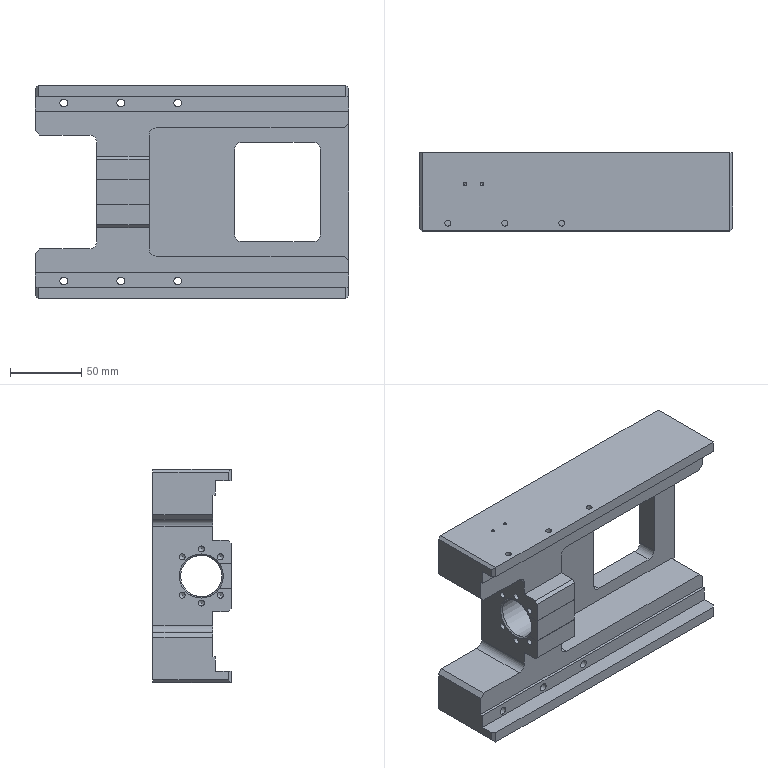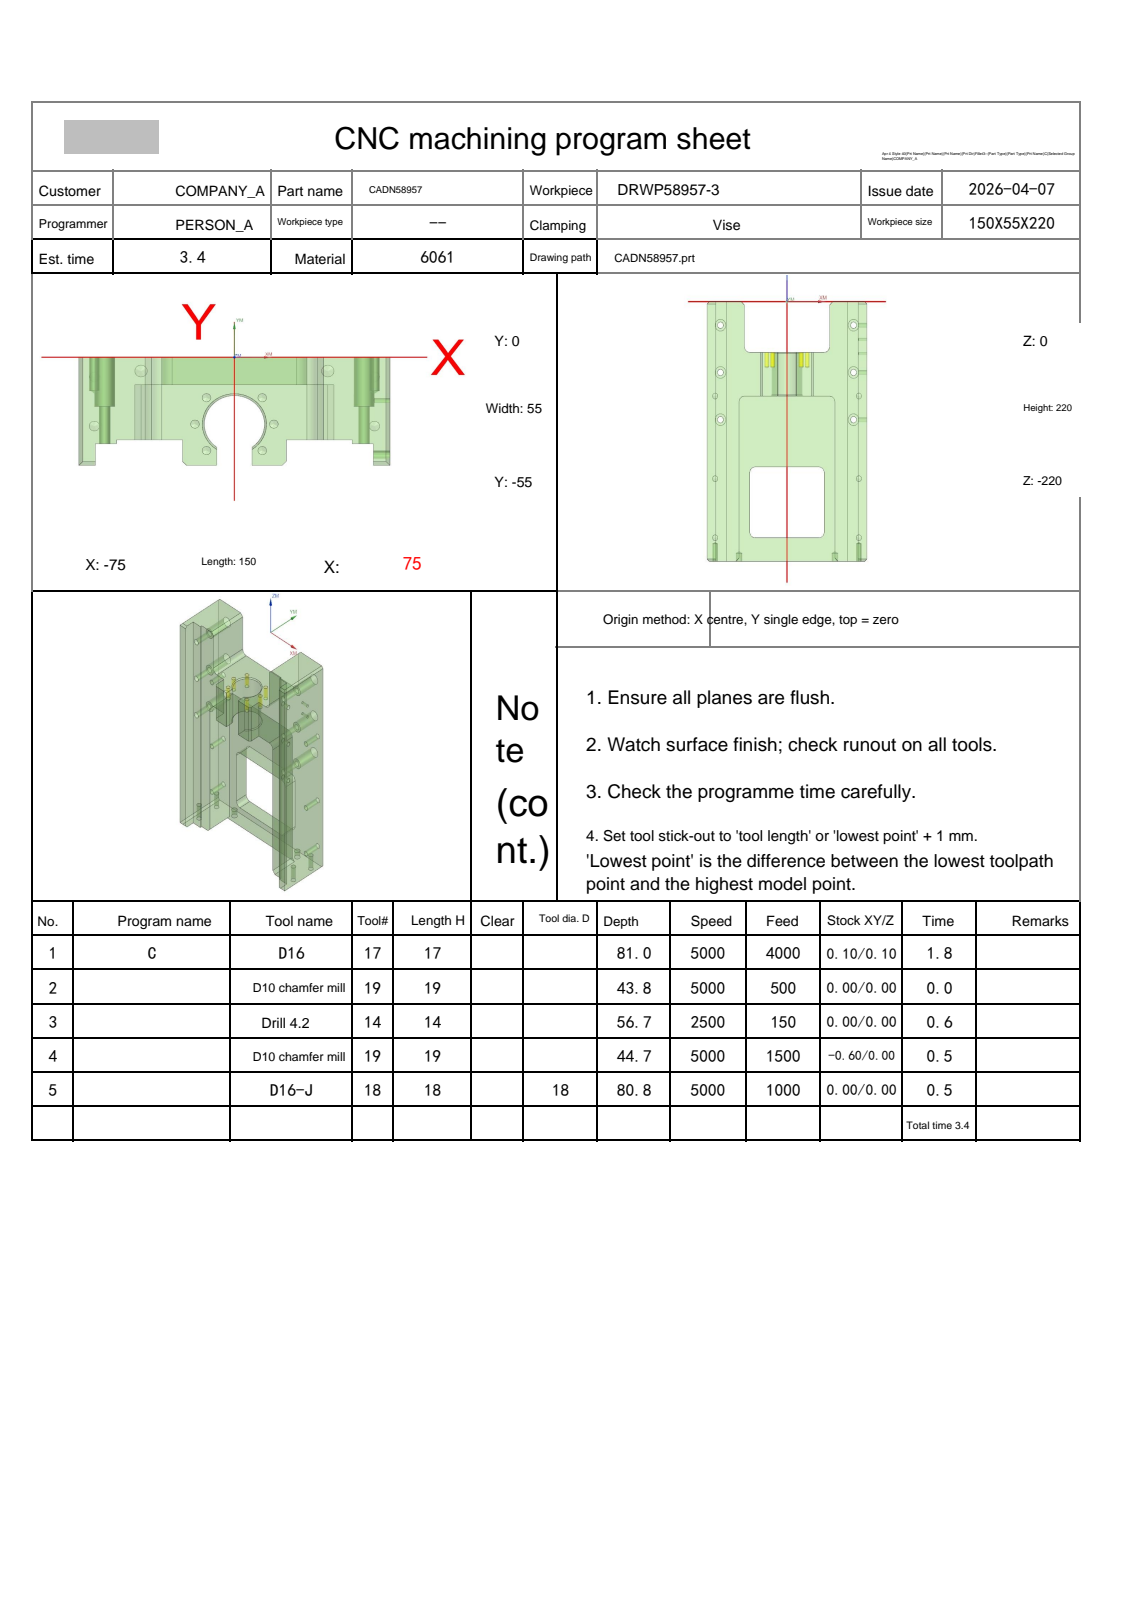NC program | NX | posted by the shop | part box 220 x 55 x 150 mm
Whole program:
%
O0001
(Machine time: 4.32 MIN)
(===Total Tool:4===)
(T17=D16    D=16.  R=0.   D-  H17 Z=-81.  )
(T19=D10 chamfer mill D=10.  R=0.   D-  H19 Z=-44.7 )
(T14=drill 4.2  D=4.2  DR_a=118 D-  H14 Z=-56.66)
(T18=D16-J  D=16.  R=0.   D18 H18 Z=-80.8 )
G80 G90 G17 G49 G40
G91 G28 Z0
M01
N1 T17 M06
(D16  D=16. R=0. H=17 ce=0.10 di=0.10)
G00 G90 G54 X13.345 Y-71.1 M03 S5000
G43 H17 Z20.
M08
Z-43.594
G01 X2.972 Y-60.728 F4000.
X2.772 Y-60.528
G02 X.4 Y-54.8 I5.728 J5.728
G01 Y-46.287
G02 X3.908 Y-39.522 I8.293 J-.008
G03 X6.765 Y-34. I-3.908 J5.522
X0.0 Y-27.235 I-6.765 J0.0
X-6.765 Y-34. I0.0 J-6.765
X-3.876 Y-39.544 I6.765 J0.0
G02 X-.4 Y-46.28 I-4.787 J-6.735
G01 Y-46.287
Y-54.8
G02 X-2.772 Y-60.528 I-8.1 J0.0
G01 X-2.972 Y-60.728
X-13.345 Y-71.1
G00 Z-44.188
G01 X-2.972 Y-60.728
X-2.772 Y-60.528
G03 X-.4 Y-54.8 I-5.728 J5.728
G01 Y-45.747
G03 X-3.752 Y-39.185 I-8.1 J0.0
G02 X-6.4 Y-34. I3.752 J5.185
X0.0 Y-27.6 I6.4 J0.0
X6.4 Y-34. I0.0 J-6.4
X3.752 Y-39.185 I-6.4 J0.0
G03 X.4 Y-45.747 I4.748 J-6.562
G01 Y-54.8
G03 X2.772 Y-60.528 I8.1 J0.0
G01 X2.972 Y-60.728
X13.345 Y-71.1
G00 Z-44.781
G01 X2.972 Y-60.728
X2.772 Y-60.528
G02 X.4 Y-54.8 I5.728 J5.728
G01 Y-45.747
G02 X3.752 Y-39.185 I8.1 J0.0
G03 X6.4 Y-34. I-3.752 J5.185
X0.0 Y-27.6 I-6.4 J0.0
X-6.4 Y-34. I0.0 J-6.4
X-3.752 Y-39.185 I6.4 J0.0
G02 X-.4 Y-45.747 I-4.748 J-6.562
G01 Y-54.8
G02 X-2.772 Y-60.528 I-8.1 J0.0
G01 X-2.972 Y-60.728
X-13.345 Y-71.1
G00 Z-45.375
G01 X-2.972 Y-60.728
X-2.772 Y-60.528
G03 X-.4 Y-54.8 I-5.728 J5.728
G01 Y-45.747
G03 X-3.752 Y-39.185 I-8.1 J0.0
G02 X-6.4 Y-34. I3.752 J5.185
X0.0 Y-27.6 I6.4 J0.0
X6.4 Y-34. I0.0 J-6.4
X3.752 Y-39.185 I-6.4 J0.0
G03 X.4 Y-45.747 I4.748 J-6.562
G01 Y-54.8
G03 X2.772 Y-60.528 I8.1 J0.0
G01 X2.972 Y-60.728
X13.345 Y-71.1
G00 Z-45.969
G01 X2.972 Y-60.728
X2.772 Y-60.528
G02 X.4 Y-54.8 I5.728 J5.728
G01 Y-45.747
G02 X3.752 Y-39.185 I8.1 J0.0
G03 X6.4 Y-34. I-3.752 J5.185
X0.0 Y-27.6 I-6.4 J0.0
X-6.4 Y-34. I0.0 J-6.4
X-3.752 Y-39.185 I6.4 J0.0
G02 X-.4 Y-45.747 I-4.748 J-6.562
G01 Y-54.8
G02 X-2.772 Y-60.528 I-8.1 J0.0
G01 X-2.972 Y-60.728
X-13.345 Y-71.1
G00 Z-46.563
G01 X-2.972 Y-60.728
X-2.772 Y-60.528
G03 X-.4 Y-54.8 I-5.728 J5.728
G01 Y-45.747
G03 X-3.752 Y-39.185 I-8.1 J0.0
G02 X-6.4 Y-34. I3.752 J5.185
X0.0 Y-27.6 I6.4 J0.0
X6.4 Y-34. I0.0 J-6.4
X3.752 Y-39.185 I-6.4 J0.0
G03 X.4 Y-45.747 I4.748 J-6.562
G01 Y-54.8
G03 X2.772 Y-60.528 I8.1 J0.0
G01 X2.972 Y-60.728
X13.345 Y-71.1
G00 Z-47.156
G01 X2.972 Y-60.728
X2.772 Y-60.528
G02 X.4 Y-54.8 I5.728 J5.728
G01 Y-45.747
G02 X3.752 Y-39.185 I8.1 J0.0
G03 X6.4 Y-34. I-3.752 J5.185
X0.0 Y-27.6 I-6.4 J0.0
X-6.4 Y-34. I0.0 J-6.4
X-3.752 Y-39.185 I6.4 J0.0
G02 X-.4 Y-45.747 I-4.748 J-6.562
G01 Y-54.8
G02 X-2.772 Y-60.528 I-8.1 J0.0
G01 X-2.972 Y-60.728
X-13.345 Y-71.1
G00 Z-47.75
G01 X-2.972 Y-60.728
X-2.772 Y-60.528
G03 X-.4 Y-54.8 I-5.728 J5.728
G01 Y-45.747
G03 X-3.752 Y-39.185 I-8.1 J0.0
G02 X-6.4 Y-34. I3.752 J5.185
X0.0 Y-27.6 I6.4 J0.0
X6.4 Y-34. I0.0 J-6.4
X3.752 Y-39.185 I-6.4 J0.0
G03 X.4 Y-45.747 I4.748 J-6.562
G01 Y-54.8
G03 X2.772 Y-60.528 I8.1 J0.0
G01 X2.972 Y-60.728
X13.345 Y-71.1
G00 Z-48.344
G01 X2.972 Y-60.728
X2.772 Y-60.528
G02 X.4 Y-54.8 I5.728 J5.728
G01 Y-45.747
G02 X3.752 Y-39.185 I8.1 J0.0
G03 X6.4 Y-34. I-3.752 J5.185
X0.0 Y-27.6 I-6.4 J0.0
X-6.4 Y-34. I0.0 J-6.4
X-3.752 Y-39.185 I6.4 J0.0
G02 X-.4 Y-45.747 I-4.748 J-6.562
G01 Y-54.8
G02 X-2.772 Y-60.528 I-8.1 J0.0
G01 X-2.972 Y-60.728
X-13.345 Y-71.1
G00 Z-48.938
G01 X-2.972 Y-60.728
X-2.772 Y-60.528
G03 X-.4 Y-54.8 I-5.728 J5.728
G01 Y-45.747
G03 X-3.752 Y-39.185 I-8.1 J0.0
G02 X-6.4 Y-34. I3.752 J5.185
X0.0 Y-27.6 I6.4 J0.0
X6.4 Y-34. I0.0 J-6.4
X3.752 Y-39.185 I-6.4 J0.0
G03 X.4 Y-45.747 I4.748 J-6.562
G01 Y-54.8
G03 X2.772 Y-60.528 I8.1 J0.0
G01 X2.972 Y-60.728
X13.345 Y-71.1
G00 Z-49.531
G01 X2.972 Y-60.728
X2.772 Y-60.528
G02 X.4 Y-54.8 I5.728 J5.728
G01 Y-45.747
G02 X3.752 Y-39.185 I8.1 J0.0
G03 X6.4 Y-34. I-3.752 J5.185
X0.0 Y-27.6 I-6.4 J0.0
X-6.4 Y-34. I0.0 J-6.4
X-3.752 Y-39.185 I6.4 J0.0
G02 X-.4 Y-45.747 I-4.748 J-6.562
G01 Y-54.8
G02 X-2.772 Y-60.528 I-8.1 J0.0
G01 X-2.972 Y-60.728
X-13.345 Y-71.1
G00 Z-50.125
G01 X-2.972 Y-60.728
X-2.772 Y-60.528
G03 X-.4 Y-54.8 I-5.728 J5.728
G01 Y-45.747
G03 X-3.752 Y-39.185 I-8.1 J0.0
G02 X-6.4 Y-34. I3.752 J5.185
X0.0 Y-27.6 I6.4 J0.0
X6.4 Y-34. I0.0 J-6.4
X3.752 Y-39.185 I-6.4 J0.0
G03 X.4 Y-45.747 I4.748 J-6.562
G01 Y-54.8
G03 X2.772 Y-60.528 I8.1 J0.0
G01 X2.972 Y-60.728
X13.345 Y-71.1
G00 Z-50.719
G01 X2.972 Y-60.728
X2.772 Y-60.528
G02 X.4 Y-54.8 I5.728 J5.728
G01 Y-45.747
G02 X3.752 Y-39.185 I8.1 J0.0
G03 X6.4 Y-34. I-3.752 J5.185
X0.0 Y-27.6 I-6.4 J0.0
X-6.4 Y-34. I0.0 J-6.4
X-3.752 Y-39.185 I6.4 J0.0
G02 X-.4 Y-45.747 I-4.748 J-6.562
G01 Y-54.8
G02 X-2.772 Y-60.528 I-8.1 J0.0
G01 X-2.972 Y-60.728
X-13.345 Y-71.1
G00 Z-51.313
G01 X-2.972 Y-60.728
X-2.772 Y-60.528
G03 X-.4 Y-54.8 I-5.728 J5.728
G01 Y-45.747
G03 X-3.752 Y-39.185 I-8.1 J0.0
G02 X-6.4 Y-34. I3.752 J5.185
X0.0 Y-27.6 I6.4 J0.0
X6.4 Y-34. I0.0 J-6.4
X3.752 Y-39.185 I-6.4 J0.0
G03 X.4 Y-45.747 I4.748 J-6.562
G01 Y-54.8
G03 X2.772 Y-60.528 I8.1 J0.0
G01 X2.972 Y-60.728
X13.345 Y-71.1
G00 Z-51.906
G01 X2.972 Y-60.728
X2.772 Y-60.528
G02 X.4 Y-54.8 I5.728 J5.728
G01 Y-45.747
G02 X3.752 Y-39.185 I8.1 J0.0
G03 X6.4 Y-34. I-3.752 J5.185
X0.0 Y-27.6 I-6.4 J0.0
X-6.4 Y-34. I0.0 J-6.4
X-3.752 Y-39.185 I6.4 J0.0
G02 X-.4 Y-45.747 I-4.748 J-6.562
G01 Y-54.8
G02 X-2.772 Y-60.528 I-8.1 J0.0
G01 X-2.972 Y-60.728
X-13.345 Y-71.1
G00 Z-52.5
G01 X-2.972 Y-60.728
X-2.772 Y-60.528
G03 X-.4 Y-54.8 I-5.728 J5.728
G01 Y-45.747
G03 X-3.752 Y-39.185 I-8.1 J0.0
G02 X-6.4 Y-34. I3.752 J5.185
X0.0 Y-27.6 I6.4 J0.0
X6.4 Y-34. I0.0 J-6.4
X3.752 Y-39.185 I-6.4 J0.0
G03 X.4 Y-45.747 I4.748 J-6.562
G01 Y-54.8
G03 X2.772 Y-60.528 I8.1 J0.0
G01 X2.972 Y-60.728
X13.345 Y-71.1
G00 Z-53.094
G01 X2.972 Y-60.728
X2.772 Y-60.528
G02 X.4 Y-54.8 I5.728 J5.728
G01 Y-45.747
G02 X3.752 Y-39.185 I8.1 J0.0
G03 X6.4 Y-34. I-3.752 J5.185
X0.0 Y-27.6 I-6.4 J0.0
X-6.4 Y-34. I0.0 J-6.4
X-3.752 Y-39.185 I6.4 J0.0
G02 X-.4 Y-45.747 I-4.748 J-6.562
G01 Y-54.8
G02 X-2.772 Y-60.528 I-8.1 J0.0
G01 X-2.972 Y-60.728
X-13.345 Y-71.1
G00 Z-53.688
G01 X-2.972 Y-60.728
X-2.772 Y-60.528
G03 X-.4 Y-54.8 I-5.728 J5.728
G01 Y-45.747
G03 X-3.752 Y-39.185 I-8.1 J0.0
G02 X-6.4 Y-34. I3.752 J5.185
X0.0 Y-27.6 I6.4 J0.0
X6.4 Y-34. I0.0 J-6.4
X3.752 Y-39.185 I-6.4 J0.0
G03 X.4 Y-45.747 I4.748 J-6.562
G01 Y-54.8
G03 X2.772 Y-60.528 I8.1 J0.0
G01 X2.972 Y-60.728
X13.345 Y-71.1
G00 Z-54.281
G01 X2.972 Y-60.728
X2.772 Y-60.528
G02 X.4 Y-54.8 I5.728 J5.728
G01 Y-45.747
G02 X3.752 Y-39.185 I8.1 J0.0
G03 X6.4 Y-34. I-3.752 J5.185
X0.0 Y-27.6 I-6.4 J0.0
X-6.4 Y-34. I0.0 J-6.4
X-3.752 Y-39.185 I6.4 J0.0
G02 X-.4 Y-45.747 I-4.748 J-6.562
G01 Y-54.8
G02 X-2.772 Y-60.528 I-8.1 J0.0
G01 X-2.972 Y-60.728
X-13.345 Y-71.1
G00 Z-54.875
G01 X-2.972 Y-60.728
X-2.772 Y-60.528
G03 X-.4 Y-54.8 I-5.728 J5.728
G01 Y-45.747
G03 X-3.752 Y-39.185 I-8.1 J0.0
G02 X-6.4 Y-34. I3.752 J5.185
X0.0 Y-27.6 I6.4 J0.0
X6.4 Y-34. I0.0 J-6.4
X3.752 Y-39.185 I-6.4 J0.0
G03 X.4 Y-45.747 I4.748 J-6.562
G01 Y-54.8
G03 X2.772 Y-60.528 I8.1 J0.0
G01 X2.972 Y-60.728
X13.345 Y-71.1
G00 Z-55.469
G01 X2.972 Y-60.728
X2.772 Y-60.528
G02 X.4 Y-54.8 I5.728 J5.728
G01 Y-45.747
G02 X3.752 Y-39.185 I8.1 J0.0
G03 X6.4 Y-34. I-3.752 J5.185
X0.0 Y-27.6 I-6.4 J0.0
X-6.4 Y-34. I0.0 J-6.4
X-3.752 Y-39.185 I6.4 J0.0
G02 X-.4 Y-45.747 I-4.748 J-6.562
G01 Y-54.8
G02 X-2.772 Y-60.528 I-8.1 J0.0
G01 X-2.972 Y-60.728
X-13.345 Y-71.1
G00 Z-56.063
G01 X-2.972 Y-60.728
X-2.772 Y-60.528
G03 X-.4 Y-54.8 I-5.728 J5.728
G01 Y-45.747
G03 X-3.752 Y-39.185 I-8.1 J0.0
G02 X-6.4 Y-34. I3.752 J5.185
X0.0 Y-27.6 I6.4 J0.0
X6.4 Y-34. I0.0 J-6.4
X3.752 Y-39.185 I-6.4 J0.0
G03 X.4 Y-45.747 I4.748 J-6.562
G01 Y-54.8
G03 X2.772 Y-60.528 I8.1 J0.0
G01 X2.972 Y-60.728
X13.345 Y-71.1
G00 Z-56.656
G01 X2.972 Y-60.728
X2.772 Y-60.528
G02 X.4 Y-54.8 I5.728 J5.728
G01 Y-45.747
G02 X3.752 Y-39.185 I8.1 J0.0
G03 X6.4 Y-34. I-3.752 J5.185
X0.0 Y-27.6 I-6.4 J0.0
X-6.4 Y-34. I0.0 J-6.4
X-3.752 Y-39.185 I6.4 J0.0
G02 X-.4 Y-45.747 I-4.748 J-6.562
G01 Y-54.8
G02 X-2.772 Y-60.528 I-8.1 J0.0
G01 X-2.972 Y-60.728
X-13.345 Y-71.1
G00 Z-57.25
G01 X-2.972 Y-60.728
X-2.772 Y-60.528
G03 X-.4 Y-54.8 I-5.728 J5.728
G01 Y-45.747
G03 X-3.752 Y-39.185 I-8.1 J0.0
G02 X-6.4 Y-34. I3.752 J5.185
X0.0 Y-27.6 I6.4 J0.0
X6.4 Y-34. I0.0 J-6.4
X3.752 Y-39.185 I-6.4 J0.0
G03 X.4 Y-45.747 I4.748 J-6.562
G01 Y-54.8
G03 X2.772 Y-60.528 I8.1 J0.0
G01 X2.972 Y-60.728
X13.345 Y-71.1
G00 Z-57.844
G01 X2.972 Y-60.728
X2.772 Y-60.528
G02 X.4 Y-54.8 I5.728 J5.728
G01 Y-45.747
G02 X3.752 Y-39.185 I8.1 J0.0
G03 X6.4 Y-34. I-3.752 J5.185
X0.0 Y-27.6 I-6.4 J0.0
X-6.4 Y-34. I0.0 J-6.4
X-3.752 Y-39.185 I6.4 J0.0
G02 X-.4 Y-45.747 I-4.748 J-6.562
G01 Y-54.8
G02 X-2.772 Y-60.528 I-8.1 J0.0
G01 X-2.972 Y-60.728
X-13.345 Y-71.1
G00 Z-58.438
G01 X-2.972 Y-60.728
X-2.772 Y-60.528
G03 X-.4 Y-54.8 I-5.728 J5.728
G01 Y-45.747
G03 X-3.752 Y-39.185 I-8.1 J0.0
G02 X-6.4 Y-34. I3.752 J5.185
X0.0 Y-27.6 I6.4 J0.0
X6.4 Y-34. I0.0 J-6.4
X3.752 Y-39.185 I-6.4 J0.0
G03 X.4 Y-45.747 I4.748 J-6.562
G01 Y-54.8
G03 X2.772 Y-60.528 I8.1 J0.0
G01 X2.972 Y-60.728
X13.345 Y-71.1
G00 Z-59.031
G01 X2.972 Y-60.728
X2.772 Y-60.528
G02 X.4 Y-54.8 I5.728 J5.728
G01 Y-45.747
G02 X3.752 Y-39.185 I8.1 J0.0
G03 X6.4 Y-34. I-3.752 J5.185
X0.0 Y-27.6 I-6.4 J0.0
X-6.4 Y-34. I0.0 J-6.4
X-3.752 Y-39.185 I6.4 J0.0
G02 X-.4 Y-45.747 I-4.748 J-6.562
G01 Y-54.8
G02 X-2.772 Y-60.528 I-8.1 J0.0
G01 X-2.972 Y-60.728
X-13.345 Y-71.1
G00 Z-59.625
G01 X-2.972 Y-60.728
X-2.772 Y-60.528
G03 X-.4 Y-54.8 I-5.728 J5.728
G01 Y-45.747
G03 X-3.752 Y-39.185 I-8.1 J0.0
G02 X-6.4 Y-34. I3.752 J5.185
X0.0 Y-27.6 I6.4 J0.0
X6.4 Y-34. I0.0 J-6.4
X3.752 Y-39.185 I-6.4 J0.0
G03 X.4 Y-45.747 I4.748 J-6.562
G01 Y-54.8
G03 X2.772 Y-60.528 I8.1 J0.0
G01 X2.972 Y-60.728
X13.345 Y-71.1
G00 Z-60.219
G01 X2.972 Y-60.728
X2.772 Y-60.528
G02 X.4 Y-54.8 I5.728 J5.728
G01 Y-45.747
G02 X3.752 Y-39.185 I8.1 J0.0
G03 X6.4 Y-34. I-3.752 J5.185
X0.0 Y-27.6 I-6.4 J0.0
X-6.4 Y-34. I0.0 J-6.4
X-3.752 Y-39.185 I6.4 J0.0
G02 X-.4 Y-45.747 I-4.748 J-6.562
G01 Y-54.8
G02 X-2.772 Y-60.528 I-8.1 J0.0
G01 X-2.972 Y-60.728
X-13.345 Y-71.1
G00 Z-60.813
G01 X-2.972 Y-60.728
X-2.772 Y-60.528
G03 X-.4 Y-54.8 I-5.728 J5.728
G01 Y-45.747
G03 X-3.752 Y-39.185 I-8.1 J0.0
G02 X-6.4 Y-34. I3.752 J5.185
X0.0 Y-27.6 I6.4 J0.0
X6.4 Y-34. I0.0 J-6.4
X3.752 Y-39.185 I-6.4 J0.0
G03 X.4 Y-45.747 I4.748 J-6.562
G01 Y-54.8
G03 X2.772 Y-60.528 I8.1 J0.0
G01 X2.972 Y-60.728
X13.345 Y-71.1
G00 Z-61.406
G01 X2.972 Y-60.728
X2.772 Y-60.528
G02 X.4 Y-54.8 I5.728 J5.728
G01 Y-45.747
G02 X3.752 Y-39.185 I8.1 J0.0
G03 X6.4 Y-34. I-3.752 J5.185
X0.0 Y-27.6 I-6.4 J0.0
X-6.4 Y-34. I0.0 J-6.4
X-3.752 Y-39.185 I6.4 J0.0
G02 X-.4 Y-45.747 I-4.748 J-6.562
G01 Y-54.8
G02 X-2.772 Y-60.528 I-8.1 J0.0
G01 X-2.972 Y-60.728
X-13.345 Y-71.1
G00 Z-62.
G01 X-2.972 Y-60.728
X-2.772 Y-60.528
G03 X-.4 Y-54.8 I-5.728 J5.728
G01 Y-45.747
G03 X-3.752 Y-39.185 I-8.1 J0.0
G02 X-6.4 Y-34. I3.752 J5.185
X0.0 Y-27.6 I6.4 J0.0
X6.4 Y-34. I0.0 J-6.4
X3.752 Y-39.185 I-6.4 J0.0
G03 X.4 Y-45.747 I4.748 J-6.562
G01 Y-54.8
G03 X2.772 Y-60.528 I8.1 J0.0
G01 X2.972 Y-60.728
X13.345 Y-71.1
G00 Z-62.594
G01 X2.972 Y-60.728
X2.772 Y-60.528
G02 X.4 Y-54.8 I5.728 J5.728
G01 Y-45.747
G02 X3.752 Y-39.185 I8.1 J0.0
G03 X6.4 Y-34. I-3.752 J5.185
X0.0 Y-27.6 I-6.4 J0.0
X-6.4 Y-34. I0.0 J-6.4
X-3.752 Y-39.185 I6.4 J0.0
G02 X-.4 Y-45.747 I-4.748 J-6.562
G01 Y-54.8
G02 X-2.772 Y-60.528 I-8.1 J0.0
G01 X-2.972 Y-60.728
X-13.345 Y-71.1
G00 Z-63.188
G01 X-2.972 Y-60.728
X-2.772 Y-60.528
G03 X-.4 Y-54.8 I-5.728 J5.728
G01 Y-45.747
G03 X-3.752 Y-39.185 I-8.1 J0.0
G02 X-6.4 Y-34. I3.752 J5.185
X0.0 Y-27.6 I6.4 J0.0
X6.4 Y-34. I0.0 J-6.4
X3.752 Y-39.185 I-6.4 J0.0
G03 X.4 Y-45.747 I4.748 J-6.562
G01 Y-54.8
G03 X2.772 Y-60.528 I8.1 J0.0
G01 X2.972 Y-60.728
X13.345 Y-71.1
G00 Z-63.781
G01 X2.972 Y-60.728
X2.772 Y-60.528
G02 X.4 Y-54.8 I5.728 J5.728
G01 Y-45.747
G02 X3.752 Y-39.185 I8.1 J0.0
G03 X6.4 Y-34. I-3.752 J5.185
X0.0 Y-27.6 I-6.4 J0.0
X-6.4 Y-34. I0.0 J-6.4
X-3.752 Y-39.185 I6.4 J0.0
G02 X-.4 Y-45.747 I-4.748 J-6.562
G01 Y-54.8
G02 X-2.772 Y-60.528 I-8.1 J0.0
G01 X-2.972 Y-60.728
X-13.345 Y-71.1
G00 Z-64.375
G01 X-2.972 Y-60.728
X-2.772 Y-60.528
G03 X-.4 Y-54.8 I-5.728 J5.728
G01 Y-45.747
G03 X-3.752 Y-39.185 I-8.1 J0.0
G02 X-6.4 Y-34. I3.752 J5.185
X0.0 Y-27.6 I6.4 J0.0
X6.4 Y-34. I0.0 J-6.4
X3.752 Y-39.185 I-6.4 J0.0
G03 X.4 Y-45.747 I4.748 J-6.562
G01 Y-54.8
G03 X2.772 Y-60.528 I8.1 J0.0
G01 X2.972 Y-60.728
X13.345 Y-71.1
G00 Z-64.969
G01 X2.972 Y-60.728
X2.772 Y-60.528
G02 X.4 Y-54.8 I5.728 J5.728
G01 Y-45.747
G02 X3.752 Y-39.185 I8.1 J0.0
G03 X6.4 Y-34. I-3.752 J5.185
X0.0 Y-27.6 I-6.4 J0.0
X-6.4 Y-34. I0.0 J-6.4
X-3.752 Y-39.185 I6.4 J0.0
G02 X-.4 Y-45.747 I-4.748 J-6.562
G01 Y-54.8
G02 X-2.772 Y-60.528 I-8.1 J0.0
G01 X-2.972 Y-60.728
X-13.345 Y-71.1
G00 Z-65.563
G01 X-2.972 Y-60.728
X-2.772 Y-60.528
G03 X-.4 Y-54.8 I-5.728 J5.728
G01 Y-45.747
G03 X-3.752 Y-39.185 I-8.1 J0.0
G02 X-6.4 Y-34. I3.752 J5.185
X0.0 Y-27.6 I6.4 J0.0
X6.4 Y-34. I0.0 J-6.4
X3.752 Y-39.185 I-6.4 J0.0
G03 X.4 Y-45.747 I4.748 J-6.562
G01 Y-54.8
G03 X2.772 Y-60.528 I8.1 J0.0
G01 X2.972 Y-60.728
X13.345 Y-71.1
G00 Z-66.156
G01 X2.972 Y-60.728
X2.772 Y-60.528
G02 X.4 Y-54.8 I5.728 J5.728
G01 Y-45.747
G02 X3.752 Y-39.185 I8.1 J0.0
G03 X6.4 Y-34. I-3.752 J5.185
X0.0 Y-27.6 I-6.4 J0.0
X-6.4 Y-34. I0.0 J-6.4
X-3.752 Y-39.185 I6.4 J0.0
G02 X-.4 Y-45.747 I-4.748 J-6.562
G01 Y-54.8
G02 X-2.772 Y-60.528 I-8.1 J0.0
G01 X-2.972 Y-60.728
X-13.345 Y-71.1
G00 Z-66.75
G01 X-2.972 Y-60.728
X-2.772 Y-60.528
G03 X-.4 Y-54.8 I-5.728 J5.728
G01 Y-45.747
G03 X-3.752 Y-39.185 I-8.1 J0.0
G02 X-6.4 Y-34. I3.752 J5.185
X0.0 Y-27.6 I6.4 J0.0
X6.4 Y-34. I0.0 J-6.4
X3.752 Y-39.185 I-6.4 J0.0
G03 X.4 Y-45.747 I4.748 J-6.562
G01 Y-54.8
G03 X2.772 Y-60.528 I8.1 J0.0
G01 X2.972 Y-60.728
X13.345 Y-71.1
G00 Z-67.344
G01 X2.972 Y-60.728
X2.772 Y-60.528
G02 X.4 Y-54.8 I5.728 J5.728
G01 Y-45.747
G02 X3.752 Y-39.185 I8.1 J0.0
G03 X6.4 Y-34. I-3.752 J5.185
X0.0 Y-27.6 I-6.4 J0.0
X-6.4 Y-34. I0.0 J-6.4
X-3.752 Y-39.185 I6.4 J0.0
G02 X-.4 Y-45.747 I-4.748 J-6.562
G01 Y-54.8
G02 X-2.772 Y-60.528 I-8.1 J0.0
G01 X-2.972 Y-60.728
X-13.345 Y-71.1
G00 Z-67.938
G01 X-2.972 Y-60.728
X-2.772 Y-60.528
G03 X-.4 Y-54.8 I-5.728 J5.728
G01 Y-45.747
G03 X-3.752 Y-39.185 I-8.1 J0.0
G02 X-6.4 Y-34. I3.752 J5.185
X0.0 Y-27.6 I6.4 J0.0
X6.4 Y-34. I0.0 J-6.4
X3.752 Y-39.185 I-6.4 J0.0
G03 X.4 Y-45.747 I4.748 J-6.562
G01 Y-54.8
G03 X2.772 Y-60.528 I8.1 J0.0
G01 X2.972 Y-60.728
X13.345 Y-71.1
G00 Z-68.531
G01 X2.972 Y-60.728
X2.772 Y-60.528
G02 X.4 Y-54.8 I5.728 J5.728
G01 Y-45.747
G02 X3.752 Y-39.185 I8.1 J0.0
G03 X6.4 Y-34. I-3.752 J5.185
X0.0 Y-27.6 I-6.4 J0.0
X-6.4 Y-34. I0.0 J-6.4
X-3.752 Y-39.185 I6.4 J0.0
G02 X-.4 Y-45.747 I-4.748 J-6.562
G01 Y-54.8
G02 X-2.772 Y-60.528 I-8.1 J0.0
G01 X-2.972 Y-60.728
X-13.345 Y-71.1
G00 Z-69.125
G01 X-2.972 Y-60.728
X-2.772 Y-60.528
G03 X-.4 Y-54.8 I-5.728 J5.728
G01 Y-45.747
G03 X-3.752 Y-39.185 I-8.1 J0.0
G02 X-6.4 Y-34. I3.752 J5.185
X0.0 Y-27.6 I6.4 J0.0
X6.4 Y-34. I0.0 J-6.4
X3.752 Y-39.185 I-6.4 J0.0
G03 X.4 Y-45.747 I4.748 J-6.562
G01 Y-54.8
G03 X2.772 Y-60.528 I8.1 J0.0
G01 X2.972 Y-60.728
X13.345 Y-71.1
G00 Z-69.719
G01 X2.972 Y-60.728
X2.772 Y-60.528
G02 X.4 Y-54.8 I5.728 J5.728
G01 Y-45.747
G02 X3.752 Y-39.185 I8.1 J0.0
G03 X6.4 Y-34. I-3.752 J5.185
X0.0 Y-27.6 I-6.4 J0.0
X-6.4 Y-34. I0.0 J-6.4
X-3.752 Y-39.185 I6.4 J0.0
G02 X-.4 Y-45.747 I-4.748 J-6.562
G01 Y-54.8
G02 X-2.772 Y-60.528 I-8.1 J0.0
G01 X-2.972 Y-60.728
X-13.345 Y-71.1
G00 Z-70.313
G01 X-2.972 Y-60.728
X-2.772 Y-60.528
G03 X-.4 Y-54.8 I-5.728 J5.728
G01 Y-45.747
G03 X-3.752 Y-39.185 I-8.1 J0.0
G02 X-6.4 Y-34. I3.752 J5.185
X0.0 Y-27.6 I6.4 J0.0
X6.4 Y-34. I0.0 J-6.4
X3.752 Y-39.185 I-6.4 J0.0
G03 X.4 Y-45.747 I4.748 J-6.562
G01 Y-54.8
G03 X2.772 Y-60.528 I8.1 J0.0
G01 X2.972 Y-60.728
X13.345 Y-71.1
G00 Z-70.906
G01 X2.972 Y-60.728
X2.772 Y-60.528
G02 X.4 Y-54.8 I5.728 J5.728
G01 Y-45.747
G02 X3.752 Y-39.185 I8.1 J0.0
G03 X6.4 Y-34. I-3.752 J5.185
X0.0 Y-27.6 I-6.4 J0.0
X-6.4 Y-34. I0.0 J-6.4
X-3.752 Y-39.185 I6.4 J0.0
G02 X-.4 Y-45.747 I-4.748 J-6.562
G01 Y-54.8
G02 X-2.772 Y-60.528 I-8.1 J0.0
G01 X-2.972 Y-60.728
X-13.345 Y-71.1
G00 Z-71.5
G01 X-2.972 Y-60.728
X-2.772 Y-60.528
G03 X-.4 Y-54.8 I-5.728 J5.728
G01 Y-45.747
G03 X-3.752 Y-39.185 I-8.1 J0.0
G02 X-6.4 Y-34. I3.752 J5.185
X0.0 Y-27.6 I6.4 J0.0
X6.4 Y-34. I0.0 J-6.4
X3.752 Y-39.185 I-6.4 J0.0
G03 X.4 Y-45.747 I4.748 J-6.562
G01 Y-54.8
G03 X2.772 Y-60.528 I8.1 J0.0
G01 X2.972 Y-60.728
X13.345 Y-71.1
G00 Z-72.094
G01 X2.972 Y-60.728
X2.772 Y-60.528
G02 X.4 Y-54.8 I5.728 J5.728
G01 Y-45.747
G02 X3.752 Y-39.185 I8.1 J0.0
G03 X6.4 Y-34. I-3.752 J5.185
X0.0 Y-27.6 I-6.4 J0.0
X-6.4 Y-34. I0.0 J-6.4
X-3.752 Y-39.185 I6.4 J0.0
G02 X-.4 Y-45.747 I-4.748 J-6.562
G01 Y-54.8
G02 X-2.772 Y-60.528 I-8.1 J0.0
G01 X-2.972 Y-60.728
X-13.345 Y-71.1
G00 Z-72.688
G01 X-2.972 Y-60.728
X-2.772 Y-60.528
G03 X-.4 Y-54.8 I-5.728 J5.728
G01 Y-45.747
G03 X-3.752 Y-39.185 I-8.1 J0.0
G02 X-6.4 Y-34. I3.752 J5.185
X0.0 Y-27.6 I6.4 J0.0
X6.4 Y-34. I0.0 J-6.4
X3.752 Y-39.185 I-6.4 J0.0
G03 X.4 Y-45.747 I4.748 J-6.562
G01 Y-54.8
G03 X2.772 Y-60.528 I8.1 J0.0
G01 X2.972 Y-60.728
X13.345 Y-71.1
G00 Z-73.281
G01 X2.972 Y-60.728
X2.772 Y-60.528
G02 X.4 Y-54.8 I5.728 J5.728
G01 Y-45.747
G02 X3.752 Y-39.185 I8.1 J0.0
G03 X6.4 Y-34. I-3.752 J5.185
X0.0 Y-27.6 I-6.4 J0.0
X-6.4 Y-34. I0.0 J-6.4
X-3.752 Y-39.185 I6.4 J0.0
G02 X-.4 Y-45.747 I-4.748 J-6.562
G01 Y-54.8
G02 X-2.772 Y-60.528 I-8.1 J0.0
G01 X-2.972 Y-60.728
X-13.345 Y-71.1
G00 Z-73.875
G01 X-2.972 Y-60.728
X-2.772 Y-60.528
G03 X-.4 Y-54.8 I-5.728 J5.728
G01 Y-45.747
G03 X-3.752 Y-39.185 I-8.1 J0.0
G02 X-6.4 Y-34. I3.752 J5.185
X0.0 Y-27.6 I6.4 J0.0
X6.4 Y-34. I0.0 J-6.4
X3.752 Y-39.185 I-6.4 J0.0
G03 X.4 Y-45.747 I4.748 J-6.562
G01 Y-54.8
G03 X2.772 Y-60.528 I8.1 J0.0
G01 X2.972 Y-60.728
X13.345 Y-71.1
G00 Z-74.469
G01 X2.972 Y-60.728
X2.772 Y-60.528
G02 X.4 Y-54.8 I5.728 J5.728
G01 Y-45.747
G02 X3.752 Y-39.185 I8.1 J0.0
G03 X6.4 Y-34. I-3.752 J5.185
X0.0 Y-27.6 I-6.4 J0.0
X-6.4 Y-34. I0.0 J-6.4
X-3.752 Y-39.185 I6.4 J0.0
G02 X-.4 Y-45.747 I-4.748 J-6.562
G01 Y-54.8
G02 X-2.772 Y-60.528 I-8.1 J0.0
G01 X-2.972 Y-60.728
X-13.345 Y-71.1
G00 Z-75.063
G01 X-2.972 Y-60.728
X-2.772 Y-60.528
G03 X-.4 Y-54.8 I-5.728 J5.728
G01 Y-45.747
G03 X-3.752 Y-39.185 I-8.1 J0.0
G02 X-6.4 Y-34. I3.752 J5.185
X0.0 Y-27.6 I6.4 J0.0
X6.4 Y-34. I0.0 J-6.4
X3.752 Y-39.185 I-6.4 J0.0
G03 X.4 Y-45.747 I4.748 J-6.562
G01 Y-54.8
G03 X2.772 Y-60.528 I8.1 J0.0
G01 X2.972 Y-60.728
X13.345 Y-71.1
G00 Z-75.656
G01 X2.972 Y-60.728
X2.772 Y-60.528
G02 X.4 Y-54.8 I5.728 J5.728
G01 Y-45.747
G02 X3.752 Y-39.185 I8.1 J0.0
G03 X6.4 Y-34. I-3.752 J5.185
X0.0 Y-27.6 I-6.4 J0.0
X-6.4 Y-34. I0.0 J-6.4
X-3.752 Y-39.185 I6.4 J0.0
G02 X-.4 Y-45.747 I-4.748 J-6.562
G01 Y-54.8
G02 X-2.772 Y-60.528 I-8.1 J0.0
G01 X-2.972 Y-60.728
X-13.345 Y-71.1
G00 Z-76.25
G01 X-2.972 Y-60.728
X-2.772 Y-60.528
G03 X-.4 Y-54.8 I-5.728 J5.728
G01 Y-45.747
G03 X-3.752 Y-39.185 I-8.1 J0.0
G02 X-6.4 Y-34. I3.752 J5.185
X0.0 Y-27.6 I6.4 J0.0
X6.4 Y-34. I0.0 J-6.4
X3.752 Y-39.185 I-6.4 J0.0
G03 X.4 Y-45.747 I4.748 J-6.562
G01 Y-54.8
G03 X2.772 Y-60.528 I8.1 J0.0
G01 X2.972 Y-60.728
X13.345 Y-71.1
G00 Z-76.844
G01 X2.972 Y-60.728
X2.772 Y-60.528
G02 X.4 Y-54.8 I5.728 J5.728
G01 Y-45.747
G02 X3.752 Y-39.185 I8.1 J0.0
G03 X6.4 Y-34. I-3.752 J5.185
X0.0 Y-27.6 I-6.4 J0.0
X-6.4 Y-34. I0.0 J-6.4
X-3.752 Y-39.185 I6.4 J0.0
G02 X-.4 Y-45.747 I-4.748 J-6.562
G01 Y-54.8
G02 X-2.772 Y-60.528 I-8.1 J0.0
G01 X-2.972 Y-60.728
X-13.345 Y-71.1
G00 Z-77.438
G01 X-2.972 Y-60.728
X-2.772 Y-60.528
G03 X-.4 Y-54.8 I-5.728 J5.728
G01 Y-45.747
G03 X-3.752 Y-39.185 I-8.1 J0.0
G02 X-6.4 Y-34. I3.752 J5.185
X0.0 Y-27.6 I6.4 J0.0
X6.4 Y-34. I0.0 J-6.4
X3.752 Y-39.185 I-6.4 J0.0
G03 X.4 Y-45.747 I4.748 J-6.562
G01 Y-54.8
G03 X2.772 Y-60.528 I8.1 J0.0
G01 X2.972 Y-60.728
X13.345 Y-71.1
G00 Z-78.031
G01 X2.972 Y-60.728
X2.772 Y-60.528
G02 X.4 Y-54.8 I5.728 J5.728
G01 Y-45.747
G02 X3.752 Y-39.185 I8.1 J0.0
G03 X6.4 Y-34. I-3.752 J5.185
X0.0 Y-27.6 I-6.4 J0.0
X-6.4 Y-34. I0.0 J-6.4
X-3.752 Y-39.185 I6.4 J0.0
G02 X-.4 Y-45.747 I-4.748 J-6.562
G01 Y-54.8
G02 X-2.772 Y-60.528 I-8.1 J0.0
G01 X-2.972 Y-60.728
X-13.345 Y-71.1
G00 Z-78.625
G01 X-2.972 Y-60.728
X-2.772 Y-60.528
G03 X-.4 Y-54.8 I-5.728 J5.728
G01 Y-45.747
G03 X-3.752 Y-39.185 I-8.1 J0.0
G02 X-6.4 Y-34. I3.752 J5.185
X0.0 Y-27.6 I6.4 J0.0
X6.4 Y-34. I0.0 J-6.4
X3.752 Y-39.185 I-6.4 J0.0
G03 X.4 Y-45.747 I4.748 J-6.562
G01 Y-54.8
G03 X2.772 Y-60.528 I8.1 J0.0
G01 X2.972 Y-60.728
X13.345 Y-71.1
G00 Z-79.219
G01 X2.972 Y-60.728
X2.772 Y-60.528
G02 X.4 Y-54.8 I5.728 J5.728
G01 Y-45.747
G02 X3.752 Y-39.185 I8.1 J0.0
G03 X6.4 Y-34. I-3.752 J5.185
X0.0 Y-27.6 I-6.4 J0.0
X-6.4 Y-34. I0.0 J-6.4
X-3.752 Y-39.185 I6.4 J0.0
G02 X-.4 Y-45.747 I-4.748 J-6.562
G01 Y-54.8
G02 X-2.772 Y-60.528 I-8.1 J0.0
G01 X-2.972 Y-60.728
X-13.345 Y-71.1
G00 Z-79.813
G01 X-2.972 Y-60.728
X-2.772 Y-60.528
G03 X-.4 Y-54.8 I-5.728 J5.728
G01 Y-45.747
G03 X-3.752 Y-39.185 I-8.1 J0.0
G02 X-6.4 Y-34. I3.752 J5.185
X0.0 Y-27.6 I6.4 J0.0
X6.4 Y-34. I0.0 J-6.4
X3.752 Y-39.185 I-6.4 J0.0
G03 X.4 Y-45.747 I4.748 J-6.562
G01 Y-54.8
G03 X2.772 Y-60.528 I8.1 J0.0
G01 X2.972 Y-60.728
X13.345 Y-71.1
G00 Z-80.406
G01 X2.972 Y-60.728
X2.772 Y-60.528
G02 X.4 Y-54.8 I5.728 J5.728
G01 Y-45.747
G02 X3.752 Y-39.185 I8.1 J0.0
G03 X6.4 Y-34. I-3.752 J5.185
X0.0 Y-27.6 I-6.4 J0.0
X-6.4 Y-34. I0.0 J-6.4
X-3.752 Y-39.185 I6.4 J0.0
G02 X-.4 Y-45.747 I-4.748 J-6.562
G01 Y-54.8
G02 X-2.772 Y-60.528 I-8.1 J0.0
G01 X-2.972 Y-60.728
X-13.345 Y-71.1
G00 Z-81.
G01 X-2.972 Y-60.728
X-2.772 Y-60.528
G03 X-.4 Y-54.8 I-5.728 J5.728
G01 Y-45.747
G03 X-3.752 Y-39.185 I-8.1 J0.0
G02 X-6.4 Y-34. I3.752 J5.185
X0.0 Y-27.6 I6.4 J0.0
X6.4 Y-34. I0.0 J-6.4
X3.752 Y-39.185 I-6.4 J0.0
G03 X.4 Y-45.747 I4.748 J-6.562
G01 Y-54.8
G03 X2.772 Y-60.528 I8.1 J0.0
G01 X2.972 Y-60.728
X13.345 Y-71.1
G00 Z20.
G91 G28 Z0.0
M05
M09
G91 G28 Z0.0
M01
N2 T19 M06
(D10 chamfer mill  D=10. R=0. H=19 ce=0.00 di=0.10)
G00 G90 G54 X13.435 Y-20.565 M03 S5000
G43 H19 Z20.
M08
G98 G81 X13.435 Y-20.565 Z-43.8 R-42. F500.
X19. Y-34.
X13.435 Y-47.435
X-13.435
X-19. Y-34.
X-13.435 Y-20.565
G80
G00 Z20.
G91 G28 Z0.0
M05
M09
G91 G28 Z0.0
M01
N3 T14 M06
(Drill 4.2 D=4.2 DR_a=118 H=14)
G00 G90 G54 X13.435 Y-20.565 M03 S2500
G43 H14 Z20.
M08
G98 G83 X13.435 Y-20.565 Z-56.662 R-42. F150. Q3.
X19. Y-34.
X13.435 Y-47.435
X-13.435
X-19. Y-34.
X-13.435 Y-20.565
G80
G00 Z20.
G91 G28 Z0.0
M05
M09
G91 G28 Z0.0
M01
N4 T19 M06
(D10 chamfer mill  D=10. R=0. H=19 ce=-0.60 di=0.00)
G00 G90 G54 X-13.038 Y-47.685 M03 S5000
G43 H19 Z20.
M08
Z-43.7
G01 Z-44.2 F500.
G03 X-14.288 Y-47.35 I-1.25 J-2.165
X-14.935 Y-47.435 I0.0 J-2.5
X-13.435 Y-48.935 I1.5 J0.0
X-11.935 Y-47.435 I0.0 J1.5
X-13.435 Y-45.935 I-1.5 J0.0
X-14.935 Y-47.435 I0.0 J-1.5
X-14.288 Y-47.52 I.647 J2.415
X-13.038 Y-47.185 I0.0 J2.5
G01 Z-43.7
G00 Z20.
X-18.603 Y-34.25
Z-43.7
G01 Z-44.2
G03 X-19.853 Y-33.915 I-1.25 J-2.165
X-20.5 Y-34. I0.0 J-2.5
X-19. Y-35.5 I1.5 J0.0
X-17.5 Y-34. I0.0 J1.5
X-19. Y-32.5 I-1.5 J0.0
X-20.5 Y-34. I0.0 J-1.5
X-19.853 Y-34.085 I.647 J2.415
X-18.603 Y-33.75 I0.0 J2.5
G01 Z-43.7
G00 Z20.
X-13.038 Y-20.815
Z-43.7
G01 Z-44.2
G03 X-14.288 Y-20.48 I-1.25 J-2.165
X-14.935 Y-20.565 I0.0 J-2.5
X-13.435 Y-22.065 I1.5 J0.0
X-11.935 Y-20.565 I0.0 J1.5
X-13.435 Y-19.065 I-1.5 J0.0
X-14.935 Y-20.565 I0.0 J-1.5
X-14.288 Y-20.65 I.647 J2.415
X-13.038 Y-20.315 I0.0 J2.5
G01 Z-43.7
G00 Z20.
X13.832 Y-20.815
Z-43.7
G01 Z-44.2
G03 X12.582 Y-20.48 I-1.25 J-2.165
X11.935 Y-20.565 I0.0 J-2.5
X13.435 Y-22.065 I1.5 J0.0
X14.935 Y-20.565 I0.0 J1.5
X13.435 Y-19.065 I-1.5 J0.0
X11.935 Y-20.565 I0.0 J-1.5
X12.582 Y-20.65 I.647 J2.415
X13.832 Y-20.315 I0.0 J2.5
G01 Z-43.7
G00 Z20.
X19.397 Y-34.25
Z-43.7
G01 Z-44.2
G03 X18.147 Y-33.915 I-1.25 J-2.165
X17.5 Y-34. I0.0 J-2.5
X19. Y-35.5 I1.5 J0.0
X20.5 Y-34. I0.0 J1.5
X19. Y-32.5 I-1.5 J0.0
X17.5 Y-34. I0.0 J-1.5
X18.147 Y-34.085 I.647 J2.415
X19.397 Y-33.75 I0.0 J2.5
G01 Z-43.7
G00 Z20.
X13.832 Y-47.685
Z-43.7
G01 Z-44.2
G03 X12.582 Y-47.35 I-1.25 J-2.165
X11.935 Y-47.435 I0.0 J-2.5
X13.435 Y-48.935 I1.5 J0.0
X14.935 Y-47.435 I0.0 J1.5
X13.435 Y-45.935 I-1.5 J0.0
X11.935 Y-47.435 I0.0 J-1.5
X12.582 Y-47.52 I.647 J2.415
X13.832 Y-47.185 I0.0 J2.5
G01 Z-43.7
G00 Z20.
G00 G90 X-8.276 Y-42.411 M03 S5000
Z20.
Z-43.2
G01 Z-44.7 F500.
X-8.373 Y-42.551
G03 X-8.731 Y-43.692 I1.643 J-1.141
X-7.872 Y-45.335 I2. J0.0
G01 X-7.709 Y-45.446
X-7.625 Y-45.502
X-7.568 Y-45.54
X0.0 Y-50.503
X7.568 Y-45.54
G03 X11.378 Y-41.809 I-7.568 J11.54
X11.51 Y-41.614 I-11.378 J7.809
X11.682 Y-41.346 I-11.51 J7.614
G01 X11.742 Y-41.25
G03 X12.013 Y-40.792 I-11.742 J7.25
G01 X12.1 Y-40.636
X12.177 Y-40.492
X12.236 Y-40.381
X12.3 Y-40.257
G03 X12.488 Y-39.872 I-12.3 J6.257
X13.8 Y-34. I-12.488 J5.872
X10.242 Y-24.751 I-13.8 J0.0
X9.22 Y-23.732 I-10.242 J-9.249
X8.782 Y-23.355 I-9.22 J-10.268
G01 X8.668 Y-23.262
G03 X8.36 Y-23.02 I-8.668 J-10.738
G01 X8.221 Y-22.916
X8.116 Y-22.839
X7.996 Y-22.753
G03 X7.802 Y-22.617 I-7.996 J-11.247
G01 X7.647 Y-22.513
G03 X5.397 Y-21.299 I-7.647 J-11.487
G01 X5.273 Y-21.247
G03 X5.028 Y-21.149 I-5.273 J-12.753
G01 X4.92 Y-21.107
X4.832 Y-21.074
X4.776 Y-21.053
X4.646 Y-21.005
G03 X4.349 Y-20.903 I-4.646 J-12.995
G01 X4.183 Y-20.849
X4.116 Y-20.828
G03 X3.608 Y-20.68 I-4.116 J-13.172
X3.325 Y-20.607 I-3.608 J-13.32
X2.658 Y-20.458 I-3.325 J-13.393
X0.0 Y-20.2 I-2.658 J-13.542
X-1.514 Y-20.283 I0.0 J-13.8
X-1.981 Y-20.343 I1.514 J-13.717
X-2.333 Y-20.399 I1.981 J-13.657
X-5.735 Y-21.448 I2.333 J-13.601
X-6.618 Y-21.891 I5.735 J-12.552
X-7.092 Y-22.162 I6.618 J-12.109
X-7.613 Y-22.49 I7.092 J-11.838
G01 X-7.712 Y-22.556
X-7.856 Y-22.655
G03 X-8.201 Y-22.901 I7.856 J-11.345
X-8.394 Y-23.047 I8.201 J-11.099
G01 X-8.54 Y-23.16
G03 X-8.751 Y-23.33 I8.54 J-10.84
X-8.974 Y-23.517 I8.751 J-10.67
X-9.928 Y-24.415 I8.974 J-10.483
X-10.194 Y-24.698 I9.928 J-9.585
G01 X-10.312 Y-24.829
X-10.355 Y-24.878
G03 X-10.686 Y-25.268 I10.355 J-9.122
X-11.018 Y-25.691 I10.686 J-8.731
X-11.138 Y-25.852 I11.018 J-8.309
X-11.396 Y-26.217 I11.138 J-8.148
X-11.716 Y-26.708 I11.396 J-7.783
X-11.943 Y-27.086 I11.716 J-7.292
G01 X-11.973 Y-27.138
G03 X-12.384 Y-27.91 I11.973 J-6.862
X-13.8 Y-34. I12.384 J-6.09
X-12.879 Y-38.956 I13.8 J0.0
G01 X-12.857 Y-39.015
G03 X-7.872 Y-45.335 I12.857 J5.015
G01 X-7.709 Y-45.446
X-7.625 Y-45.502
X-7.568 Y-45.54
X-7.54 Y-45.558
G03 X-6.443 Y-45.886 I1.097 J1.672
X-4.8 Y-45.026 I0.0 J2.
G01 Z-43.2
G00 Z20.
G00 G90 X-7.8 Y-53.022 M03 S5000
Z20.
Z-40.5
G01 Y-54.8 Z-41.147 F1500.
Y-46.961 Z-44.
Y-54.8
Z-41.5
G00 Z20.
X7.8 Y-48.739
Z-40.5
G01 Y-46.961 Z-41.147
Y-54.8 Z-44.
Y-46.961
Z-41.5
G00 Z20.
G91 G28 Z0.0
M05
M09
G91 G28 Z0.0
M01
N5 T18 M06
(D16-J  D=16. R=0. H=18 ce=0.00 di=0.00)
G00 G90 G54 X8.559 Y-69.849 M03 S5000
G43 H18 Z10.005
M08
Z-50.95
G01 Z-52.45 F1000.
G41 D18
X8.7 Y-69.708
G03 X9.403 Y-68.011 I-1.697 J1.697
X8.7 Y-66.314 I-2.4 J0.0
G01 X.5 Y-58.114
Y-41.661
X3.81 Y-39.266
G03 X6.5 Y-34. I-3.81 J5.266
X0.0 Y-27.5 I-6.5 J0.0
X-6.5 Y-34. I0.0 J-6.5
X-3.81 Y-39.266 I6.5 J0.0
G01 X-.5 Y-41.661
Y-58.114
X-8.7 Y-66.314
G03 X-9.403 Y-68.011 I1.697 J-1.697
X-8.7 Y-69.708 I2.4 J0.0
G01 G40 X-8.559 Y-69.849
Z-50.95
G00 X8.559
Z-60.4
G01 Z-61.9
G41 D18
X8.7 Y-69.708
G03 X9.403 Y-68.011 I-1.697 J1.697
X8.7 Y-66.314 I-2.4 J0.0
G01 X.5 Y-58.114
Y-41.661
X3.81 Y-39.266
G03 X6.5 Y-34. I-3.81 J5.266
X0.0 Y-27.5 I-6.5 J0.0
X-6.5 Y-34. I0.0 J-6.5
X-3.81 Y-39.266 I6.5 J0.0
G01 X-.5 Y-41.661
Y-58.114
X-8.7 Y-66.314
G03 X-9.403 Y-68.011 I1.697 J-1.697
X-8.7 Y-69.708 I2.4 J0.0
G01 G40 X-8.559 Y-69.849
Z-60.4
G00 X8.559
Z-69.85
G01 Z-71.35
G41 D18
X8.7 Y-69.708
G03 X9.403 Y-68.011 I-1.697 J1.697
X8.7 Y-66.314 I-2.4 J0.0
G01 X.5 Y-58.114
Y-41.661
X3.81 Y-39.266
G03 X6.5 Y-34. I-3.81 J5.266
X0.0 Y-27.5 I-6.5 J0.0
X-6.5 Y-34. I0.0 J-6.5
X-3.81 Y-39.266 I6.5 J0.0
G01 X-.5 Y-41.661
Y-58.114
X-8.7 Y-66.314
G03 X-9.403 Y-68.011 I1.697 J-1.697
X-8.7 Y-69.708 I2.4 J0.0
G01 G40 X-8.559 Y-69.849
Z-69.85
G00 X8.559
Z-79.3
G01 Z-80.8
G41 D18
X8.7 Y-69.708
G03 X9.403 Y-68.011 I-1.697 J1.697
X8.7 Y-66.314 I-2.4 J0.0
G01 X.5 Y-58.114
Y-41.661
X3.81 Y-39.266
G03 X6.5 Y-34. I-3.81 J5.266
X0.0 Y-27.5 I-6.5 J0.0
X-6.5 Y-34. I0.0 J-6.5
X-3.81 Y-39.266 I6.5 J0.0
G01 X-.5 Y-41.661
Y-58.114
X-8.7 Y-66.314
G03 X-9.403 Y-68.011 I1.697 J-1.697
X-8.7 Y-69.708 I2.4 J0.0
G01 G40 X-8.559 Y-69.849
Z-79.3
G00 Z10.005
M05
M09
G91 G28 Z0.0
G91 G28 Y0.0
M30
%